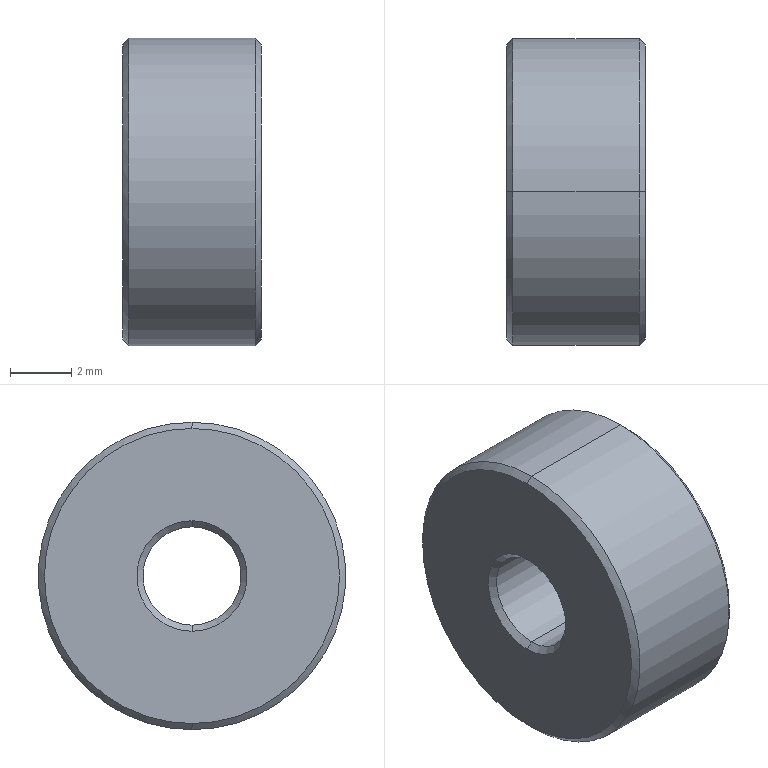Part | SolidWorks | features BaseBody 1 | 1 solid | 14 faces | box 4.5 x 10 x 10 mm | volume 315.579 mm3 | cone 8 | cylinder 4 | plane 2 | commonest cylinder face diameters 3.2 x2 10 x2
STEP:
#1=CARTESIAN_POINT('',(4.5,0.,-4.8));
#2=VERTEX_POINT('',#1);
#3=CARTESIAN_POINT('',(4.3,0.,-5.));
#4=VERTEX_POINT('',#3);
#5=CARTESIAN_POINT('',(4.5,0.,-4.8));
#6=DIRECTION('',(-0.7071,0.,-0.7071));
#7=VECTOR('',#6,1000.);
#8=LINE('',#5,#7);
#9=EDGE_CURVE('',#2,#4,#8,.T.);
#10=ORIENTED_EDGE('',*,*,#9,.F.);
#11=CARTESIAN_POINT('',(4.5,0.,4.8));
#12=VERTEX_POINT('',#11);
#13=CARTESIAN_POINT('',(4.5,0.,0.));
#14=DIRECTION('',(1.,0.,0.));
#15=DIRECTION('',(0.,0.,-1.));
#16=AXIS2_PLACEMENT_3D('',#13,#14,#15);
#17=CIRCLE('',#16,4.8);
#18=EDGE_CURVE('',#12,#2,#17,.T.);
#19=ORIENTED_EDGE('',*,*,#18,.F.);
#20=CARTESIAN_POINT('',(4.3,0.,5.));
#21=VERTEX_POINT('',#20);
#22=CARTESIAN_POINT('',(4.5,0.,4.8));
#23=DIRECTION('',(-0.7071,0.,0.7071));
#24=VECTOR('',#23,1000.);
#25=LINE('',#22,#24);
#26=EDGE_CURVE('',#12,#21,#25,.T.);
#27=ORIENTED_EDGE('',*,*,#26,.T.);
#28=CARTESIAN_POINT('',(4.3,0.,0.));
#29=DIRECTION('',(-1.,0.,0.));
#30=DIRECTION('',(0.,0.,-1.));
#31=AXIS2_PLACEMENT_3D('',#28,#29,#30);
#32=CIRCLE('',#31,5.);
#33=EDGE_CURVE('',#4,#21,#32,.T.);
#34=ORIENTED_EDGE('',*,*,#33,.F.);
#35=EDGE_LOOP('',(#10,#19,#27,#34));
#36=FACE_OUTER_BOUND('',#35,.T.);
#37=CARTESIAN_POINT('',(4.5,0.,0.));
#38=DIRECTION('',(-1.,0.,0.));
#39=DIRECTION('',(0.,0.,1.));
#40=AXIS2_PLACEMENT_3D('',#37,#38,#39);
#41=CONICAL_SURFACE('',#40,4.8,0.7854);
#42=ADVANCED_FACE('',(#36),#41,.T.);
#43=CARTESIAN_POINT('',(4.3,0.,1.6));
#44=VERTEX_POINT('',#43);
#45=CARTESIAN_POINT('',(4.5,0.,1.8));
#46=VERTEX_POINT('',#45);
#47=CARTESIAN_POINT('',(4.3,0.,1.6));
#48=DIRECTION('',(0.7071,0.,0.7071));
#49=VECTOR('',#48,1000.);
#50=LINE('',#47,#49);
#51=EDGE_CURVE('',#44,#46,#50,.T.);
#52=ORIENTED_EDGE('',*,*,#51,.F.);
#53=CARTESIAN_POINT('',(4.3,0.,-1.6));
#54=VERTEX_POINT('',#53);
#55=CARTESIAN_POINT('',(4.3,0.,0.));
#56=DIRECTION('',(1.,0.,0.));
#57=DIRECTION('',(0.,0.,-1.));
#58=AXIS2_PLACEMENT_3D('',#55,#56,#57);
#59=CIRCLE('',#58,1.6);
#60=EDGE_CURVE('',#54,#44,#59,.T.);
#61=ORIENTED_EDGE('',*,*,#60,.F.);
#62=CARTESIAN_POINT('',(4.5,0.,-1.8));
#63=VERTEX_POINT('',#62);
#64=CARTESIAN_POINT('',(4.3,0.,-1.6));
#65=DIRECTION('',(0.7071,0.,-0.7071));
#66=VECTOR('',#65,1000.);
#67=LINE('',#64,#66);
#68=EDGE_CURVE('',#54,#63,#67,.T.);
#69=ORIENTED_EDGE('',*,*,#68,.T.);
#70=CARTESIAN_POINT('',(4.5,0.,0.));
#71=DIRECTION('',(-1.,0.,0.));
#72=DIRECTION('',(0.,0.,-1.));
#73=AXIS2_PLACEMENT_3D('',#70,#71,#72);
#74=CIRCLE('',#73,1.8);
#75=EDGE_CURVE('',#46,#63,#74,.T.);
#76=ORIENTED_EDGE('',*,*,#75,.F.);
#77=EDGE_LOOP('',(#52,#61,#69,#76));
#78=FACE_OUTER_BOUND('',#77,.T.);
#79=CARTESIAN_POINT('',(4.3,0.,0.));
#80=DIRECTION('',(1.,0.,0.));
#81=DIRECTION('',(0.,0.,-1.));
#82=AXIS2_PLACEMENT_3D('',#79,#80,#81);
#83=CONICAL_SURFACE('',#82,1.6,0.7854);
#84=ADVANCED_FACE('',(#78),#83,.F.);
#85=CARTESIAN_POINT('',(0.2,0.,-1.6));
#86=VERTEX_POINT('',#85);
#87=CARTESIAN_POINT('',(0.,0.,-1.8));
#88=VERTEX_POINT('',#87);
#89=CARTESIAN_POINT('',(0.,0.,-1.8));
#90=DIRECTION('',(-0.7071,0.,-0.7071));
#91=VECTOR('',#90,1000.);
#92=LINE('',#89,#91);
#93=EDGE_CURVE('',#86,#88,#92,.T.);
#94=ORIENTED_EDGE('',*,*,#93,.F.);
#95=CARTESIAN_POINT('',(0.2,0.,1.6));
#96=VERTEX_POINT('',#95);
#97=CARTESIAN_POINT('',(0.2,0.,0.));
#98=DIRECTION('',(-1.,0.,0.));
#99=DIRECTION('',(0.,0.,-1.));
#100=AXIS2_PLACEMENT_3D('',#97,#98,#99);
#101=CIRCLE('',#100,1.6);
#102=EDGE_CURVE('',#96,#86,#101,.T.);
#103=ORIENTED_EDGE('',*,*,#102,.F.);
#104=CARTESIAN_POINT('',(0.,0.,1.8));
#105=VERTEX_POINT('',#104);
#106=CARTESIAN_POINT('',(0.,0.,1.8));
#107=DIRECTION('',(-0.7071,0.,0.7071));
#108=VECTOR('',#107,1000.);
#109=LINE('',#106,#108);
#110=EDGE_CURVE('',#96,#105,#109,.T.);
#111=ORIENTED_EDGE('',*,*,#110,.T.);
#112=CARTESIAN_POINT('',(0.,0.,0.));
#113=DIRECTION('',(1.,0.,0.));
#114=DIRECTION('',(0.,0.,-1.));
#115=AXIS2_PLACEMENT_3D('',#112,#113,#114);
#116=CIRCLE('',#115,1.8);
#117=EDGE_CURVE('',#88,#105,#116,.T.);
#118=ORIENTED_EDGE('',*,*,#117,.F.);
#119=EDGE_LOOP('',(#94,#103,#111,#118));
#120=FACE_OUTER_BOUND('',#119,.T.);
#121=CARTESIAN_POINT('',(0.,0.,0.));
#122=DIRECTION('',(-1.,0.,0.));
#123=DIRECTION('',(0.,0.,1.));
#124=AXIS2_PLACEMENT_3D('',#121,#122,#123);
#125=CONICAL_SURFACE('',#124,1.8,0.7854);
#126=ADVANCED_FACE('',(#120),#125,.F.);
#127=CARTESIAN_POINT('',(0.,0.,4.8));
#128=VERTEX_POINT('',#127);
#129=CARTESIAN_POINT('',(0.2,0.,5.));
#130=VERTEX_POINT('',#129);
#131=CARTESIAN_POINT('',(0.2,0.,5.));
#132=DIRECTION('',(0.7071,0.,0.7071));
#133=VECTOR('',#132,1000.);
#134=LINE('',#131,#133);
#135=EDGE_CURVE('',#128,#130,#134,.T.);
#136=ORIENTED_EDGE('',*,*,#135,.F.);
#137=CARTESIAN_POINT('',(0.,0.,-4.8));
#138=VERTEX_POINT('',#137);
#139=CARTESIAN_POINT('',(0.,0.,0.));
#140=DIRECTION('',(-1.,0.,0.));
#141=DIRECTION('',(0.,0.,-1.));
#142=AXIS2_PLACEMENT_3D('',#139,#140,#141);
#143=CIRCLE('',#142,4.8);
#144=EDGE_CURVE('',#138,#128,#143,.T.);
#145=ORIENTED_EDGE('',*,*,#144,.F.);
#146=CARTESIAN_POINT('',(0.2,0.,-5.));
#147=VERTEX_POINT('',#146);
#148=CARTESIAN_POINT('',(0.2,0.,-5.));
#149=DIRECTION('',(0.7071,0.,-0.7071));
#150=VECTOR('',#149,1000.);
#151=LINE('',#148,#150);
#152=EDGE_CURVE('',#138,#147,#151,.T.);
#153=ORIENTED_EDGE('',*,*,#152,.T.);
#154=CARTESIAN_POINT('',(0.2,0.,0.));
#155=DIRECTION('',(1.,0.,0.));
#156=DIRECTION('',(0.,0.,-1.));
#157=AXIS2_PLACEMENT_3D('',#154,#155,#156);
#158=CIRCLE('',#157,5.);
#159=EDGE_CURVE('',#130,#147,#158,.T.);
#160=ORIENTED_EDGE('',*,*,#159,.F.);
#161=EDGE_LOOP('',(#136,#145,#153,#160));
#162=FACE_OUTER_BOUND('',#161,.T.);
#163=CARTESIAN_POINT('',(0.2,0.,0.));
#164=DIRECTION('',(1.,0.,0.));
#165=DIRECTION('',(0.,0.,-1.));
#166=AXIS2_PLACEMENT_3D('',#163,#164,#165);
#167=CONICAL_SURFACE('',#166,5.,0.7854);
#168=ADVANCED_FACE('',(#162),#167,.T.);
#169=CARTESIAN_POINT('',(4.5,0.,-1.6));
#170=DIRECTION('',(-1.,0.,0.));
#171=VECTOR('',#170,1000.);
#172=LINE('',#169,#171);
#173=EDGE_CURVE('',#54,#86,#172,.T.);
#174=ORIENTED_EDGE('',*,*,#173,.F.);
#175=ORIENTED_EDGE('',*,*,#60,.T.);
#176=CARTESIAN_POINT('',(4.5,0.,1.6));
#177=DIRECTION('',(-1.,0.,0.));
#178=VECTOR('',#177,1000.);
#179=LINE('',#176,#178);
#180=EDGE_CURVE('',#44,#96,#179,.T.);
#181=ORIENTED_EDGE('',*,*,#180,.T.);
#182=ORIENTED_EDGE('',*,*,#102,.T.);
#183=EDGE_LOOP('',(#174,#175,#181,#182));
#184=FACE_OUTER_BOUND('',#183,.T.);
#185=CARTESIAN_POINT('',(4.5,0.,0.));
#186=DIRECTION('',(-1.,0.,0.));
#187=DIRECTION('',(0.,0.,1.));
#188=AXIS2_PLACEMENT_3D('',#185,#186,#187);
#189=CYLINDRICAL_SURFACE('',#188,1.6);
#190=ADVANCED_FACE('',(#184),#189,.F.);
#191=CARTESIAN_POINT('',(4.5,0.,-5.));
#192=DIRECTION('',(-1.,0.,0.));
#193=VECTOR('',#192,1000.);
#194=LINE('',#191,#193);
#195=EDGE_CURVE('',#4,#147,#194,.T.);
#196=ORIENTED_EDGE('',*,*,#195,.F.);
#197=ORIENTED_EDGE('',*,*,#33,.T.);
#198=CARTESIAN_POINT('',(4.5,0.,5.));
#199=DIRECTION('',(-1.,0.,0.));
#200=VECTOR('',#199,1000.);
#201=LINE('',#198,#200);
#202=EDGE_CURVE('',#21,#130,#201,.T.);
#203=ORIENTED_EDGE('',*,*,#202,.T.);
#204=ORIENTED_EDGE('',*,*,#159,.T.);
#205=EDGE_LOOP('',(#196,#197,#203,#204));
#206=FACE_OUTER_BOUND('',#205,.T.);
#207=CARTESIAN_POINT('',(4.5,0.,0.));
#208=DIRECTION('',(-1.,0.,0.));
#209=DIRECTION('',(0.,0.,1.));
#210=AXIS2_PLACEMENT_3D('',#207,#208,#209);
#211=CYLINDRICAL_SURFACE('',#210,5.);
#212=ADVANCED_FACE('',(#206),#211,.T.);
#213=CARTESIAN_POINT('',(0.,0.,0.));
#214=DIRECTION('',(1.,0.,0.));
#215=DIRECTION('',(0.,0.,-1.));
#216=AXIS2_PLACEMENT_3D('',#213,#214,#215);
#217=CIRCLE('',#216,1.8);
#218=EDGE_CURVE('',#105,#88,#217,.T.);
#219=ORIENTED_EDGE('',*,*,#218,.T.);
#220=ORIENTED_EDGE('',*,*,#117,.T.);
#221=EDGE_LOOP('',(#219,#220));
#222=FACE_BOUND('',#221,.T.);
#223=ORIENTED_EDGE('',*,*,#144,.T.);
#224=CARTESIAN_POINT('',(0.,0.,0.));
#225=DIRECTION('',(-1.,0.,0.));
#226=DIRECTION('',(0.,0.,-1.));
#227=AXIS2_PLACEMENT_3D('',#224,#225,#226);
#228=CIRCLE('',#227,4.8);
#229=EDGE_CURVE('',#128,#138,#228,.T.);
#230=ORIENTED_EDGE('',*,*,#229,.T.);
#231=EDGE_LOOP('',(#223,#230));
#232=FACE_OUTER_BOUND('',#231,.T.);
#233=CARTESIAN_POINT('',(0.,0.,0.));
#234=DIRECTION('',(1.,0.,0.));
#235=DIRECTION('',(0.,1.,0.));
#236=AXIS2_PLACEMENT_3D('',#233,#234,#235);
#237=PLANE('',#236);
#238=ADVANCED_FACE('',(#222,#232),#237,.F.);
#239=CARTESIAN_POINT('',(4.5,0.,0.));
#240=DIRECTION('',(-1.,0.,0.));
#241=DIRECTION('',(0.,0.,-1.));
#242=AXIS2_PLACEMENT_3D('',#239,#240,#241);
#243=CIRCLE('',#242,1.8);
#244=EDGE_CURVE('',#63,#46,#243,.T.);
#245=ORIENTED_EDGE('',*,*,#244,.T.);
#246=ORIENTED_EDGE('',*,*,#75,.T.);
#247=EDGE_LOOP('',(#245,#246));
#248=FACE_BOUND('',#247,.T.);
#249=ORIENTED_EDGE('',*,*,#18,.T.);
#250=CARTESIAN_POINT('',(4.5,0.,0.));
#251=DIRECTION('',(1.,0.,0.));
#252=DIRECTION('',(0.,0.,-1.));
#253=AXIS2_PLACEMENT_3D('',#250,#251,#252);
#254=CIRCLE('',#253,4.8);
#255=EDGE_CURVE('',#2,#12,#254,.T.);
#256=ORIENTED_EDGE('',*,*,#255,.T.);
#257=EDGE_LOOP('',(#249,#256));
#258=FACE_OUTER_BOUND('',#257,.T.);
#259=CARTESIAN_POINT('',(4.5,0.,0.));
#260=DIRECTION('',(1.,0.,0.));
#261=DIRECTION('',(0.,1.,0.));
#262=AXIS2_PLACEMENT_3D('',#259,#260,#261);
#263=PLANE('',#262);
#264=ADVANCED_FACE('',(#248,#258),#263,.T.);
#265=CARTESIAN_POINT('',(4.3,0.,0.));
#266=DIRECTION('',(-1.,0.,0.));
#267=DIRECTION('',(0.,0.,-1.));
#268=AXIS2_PLACEMENT_3D('',#265,#266,#267);
#269=CIRCLE('',#268,5.);
#270=EDGE_CURVE('',#21,#4,#269,.T.);
#271=ORIENTED_EDGE('',*,*,#270,.T.);
#272=ORIENTED_EDGE('',*,*,#195,.T.);
#273=CARTESIAN_POINT('',(0.2,0.,0.));
#274=DIRECTION('',(1.,0.,0.));
#275=DIRECTION('',(0.,0.,-1.));
#276=AXIS2_PLACEMENT_3D('',#273,#274,#275);
#277=CIRCLE('',#276,5.);
#278=EDGE_CURVE('',#147,#130,#277,.T.);
#279=ORIENTED_EDGE('',*,*,#278,.T.);
#280=ORIENTED_EDGE('',*,*,#202,.F.);
#281=EDGE_LOOP('',(#271,#272,#279,#280));
#282=FACE_OUTER_BOUND('',#281,.T.);
#283=CARTESIAN_POINT('',(4.5,0.,0.));
#284=DIRECTION('',(-1.,0.,0.));
#285=DIRECTION('',(0.,0.,1.));
#286=AXIS2_PLACEMENT_3D('',#283,#284,#285);
#287=CYLINDRICAL_SURFACE('',#286,5.);
#288=ADVANCED_FACE('',(#282),#287,.T.);
#289=CARTESIAN_POINT('',(4.3,0.,0.));
#290=DIRECTION('',(1.,0.,0.));
#291=DIRECTION('',(0.,0.,-1.));
#292=AXIS2_PLACEMENT_3D('',#289,#290,#291);
#293=CIRCLE('',#292,1.6);
#294=EDGE_CURVE('',#44,#54,#293,.T.);
#295=ORIENTED_EDGE('',*,*,#294,.T.);
#296=ORIENTED_EDGE('',*,*,#173,.T.);
#297=CARTESIAN_POINT('',(0.2,0.,0.));
#298=DIRECTION('',(-1.,0.,0.));
#299=DIRECTION('',(0.,0.,-1.));
#300=AXIS2_PLACEMENT_3D('',#297,#298,#299);
#301=CIRCLE('',#300,1.6);
#302=EDGE_CURVE('',#86,#96,#301,.T.);
#303=ORIENTED_EDGE('',*,*,#302,.T.);
#304=ORIENTED_EDGE('',*,*,#180,.F.);
#305=EDGE_LOOP('',(#295,#296,#303,#304));
#306=FACE_OUTER_BOUND('',#305,.T.);
#307=CARTESIAN_POINT('',(4.5,0.,0.));
#308=DIRECTION('',(-1.,0.,0.));
#309=DIRECTION('',(0.,0.,1.));
#310=AXIS2_PLACEMENT_3D('',#307,#308,#309);
#311=CYLINDRICAL_SURFACE('',#310,1.6);
#312=ADVANCED_FACE('',(#306),#311,.F.);
#313=ORIENTED_EDGE('',*,*,#229,.F.);
#314=ORIENTED_EDGE('',*,*,#135,.T.);
#315=ORIENTED_EDGE('',*,*,#278,.F.);
#316=ORIENTED_EDGE('',*,*,#152,.F.);
#317=EDGE_LOOP('',(#313,#314,#315,#316));
#318=FACE_OUTER_BOUND('',#317,.T.);
#319=CARTESIAN_POINT('',(0.2,0.,0.));
#320=DIRECTION('',(1.,0.,0.));
#321=DIRECTION('',(0.,0.,-1.));
#322=AXIS2_PLACEMENT_3D('',#319,#320,#321);
#323=CONICAL_SURFACE('',#322,5.,0.7854);
#324=ADVANCED_FACE('',(#318),#323,.T.);
#325=ORIENTED_EDGE('',*,*,#302,.F.);
#326=ORIENTED_EDGE('',*,*,#93,.T.);
#327=ORIENTED_EDGE('',*,*,#218,.F.);
#328=ORIENTED_EDGE('',*,*,#110,.F.);
#329=EDGE_LOOP('',(#325,#326,#327,#328));
#330=FACE_OUTER_BOUND('',#329,.T.);
#331=CARTESIAN_POINT('',(0.,0.,0.));
#332=DIRECTION('',(-1.,0.,0.));
#333=DIRECTION('',(0.,0.,1.));
#334=AXIS2_PLACEMENT_3D('',#331,#332,#333);
#335=CONICAL_SURFACE('',#334,1.8,0.7854);
#336=ADVANCED_FACE('',(#330),#335,.F.);
#337=ORIENTED_EDGE('',*,*,#294,.F.);
#338=ORIENTED_EDGE('',*,*,#51,.T.);
#339=ORIENTED_EDGE('',*,*,#244,.F.);
#340=ORIENTED_EDGE('',*,*,#68,.F.);
#341=EDGE_LOOP('',(#337,#338,#339,#340));
#342=FACE_OUTER_BOUND('',#341,.T.);
#343=CARTESIAN_POINT('',(4.3,0.,0.));
#344=DIRECTION('',(1.,0.,0.));
#345=DIRECTION('',(0.,0.,-1.));
#346=AXIS2_PLACEMENT_3D('',#343,#344,#345);
#347=CONICAL_SURFACE('',#346,1.6,0.7854);
#348=ADVANCED_FACE('',(#342),#347,.F.);
#349=ORIENTED_EDGE('',*,*,#255,.F.);
#350=ORIENTED_EDGE('',*,*,#9,.T.);
#351=ORIENTED_EDGE('',*,*,#270,.F.);
#352=ORIENTED_EDGE('',*,*,#26,.F.);
#353=EDGE_LOOP('',(#349,#350,#351,#352));
#354=FACE_OUTER_BOUND('',#353,.T.);
#355=CARTESIAN_POINT('',(4.5,0.,0.));
#356=DIRECTION('',(-1.,0.,0.));
#357=DIRECTION('',(0.,0.,1.));
#358=AXIS2_PLACEMENT_3D('',#355,#356,#357);
#359=CONICAL_SURFACE('',#358,4.8,0.7854);
#360=ADVANCED_FACE('',(#354),#359,.T.);
#361=CLOSED_SHELL('',(#42,#84,#126,#168,#190,#212,#238,#264,#288,#312,#324,#336,#348,#360));
#362=MANIFOLD_SOLID_BREP('',#361);
#363=CARTESIAN_POINT('',(0.,0.,0.));
#364=DIRECTION('',(0.,0.,1.));
#365=DIRECTION('',(1.,0.,0.));
#366=AXIS2_PLACEMENT_3D('',#363,#364,#365);
#367=(LENGTH_UNIT()NAMED_UNIT(*)SI_UNIT(.MILLI.,.METRE.));
#368=UNCERTAINTY_MEASURE_WITH_UNIT(LENGTH_MEASURE(0.00001),#367,'','');
#369=(NAMED_UNIT(*)PLANE_ANGLE_UNIT()SI_UNIT($,.RADIAN.));
#370=(NAMED_UNIT(*)SI_UNIT($,.STERADIAN.)SOLID_ANGLE_UNIT());
#371=(GEOMETRIC_REPRESENTATION_CONTEXT(3)GLOBAL_UNCERTAINTY_ASSIGNED_CONTEXT((#368))GLOBAL_UNIT_ASSIGNED_CONTEXT((#367,#369,#370))REPRESENTATION_CONTEXT('',''));
#372=ADVANCED_BREP_SHAPE_REPRESENTATION('',(#362,#366),#371);